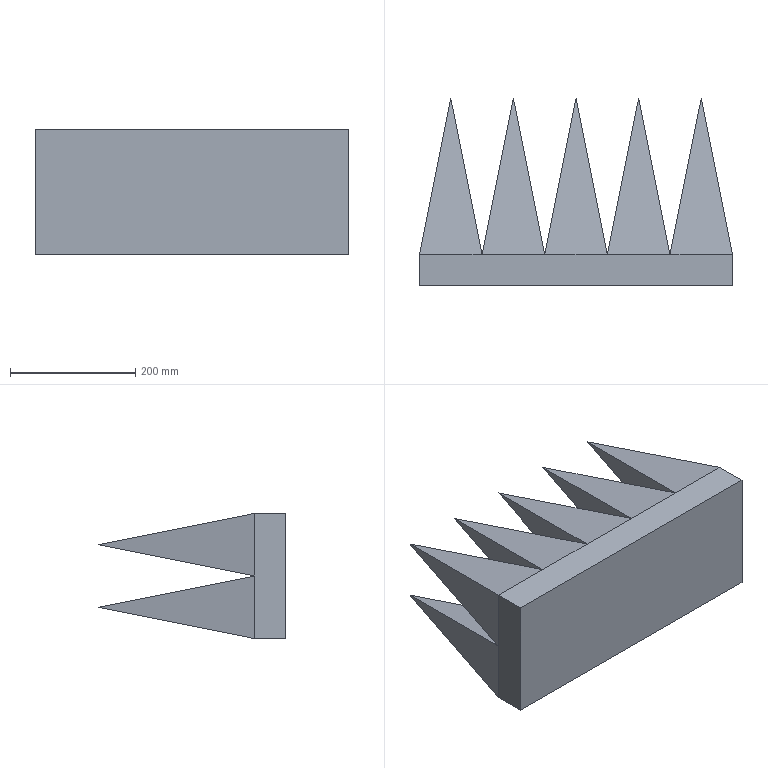Part | SolidWorks | features LPattern 2, Blend 1, Extrusion 1, ICE 1 | 1 solid | 45 faces | box 500 x 300 x 200 mm | volume 13333333 mm3 | plane 45
STEP:
#1=CARTESIAN_POINT('',(250.,50.,-50.));
#2=VERTEX_POINT('',#1);
#3=CARTESIAN_POINT('',(250.,50.,-150.));
#4=VERTEX_POINT('',#3);
#5=CARTESIAN_POINT('',(250.,50.,-50.));
#6=CARTESIAN_POINT('',(250.,50.,-83.333));
#7=CARTESIAN_POINT('',(250.,50.,-116.667));
#8=CARTESIAN_POINT('',(250.,50.,-150.));
#9=B_SPLINE_CURVE_WITH_KNOTS('',3,(#5,#6,#7,#8),.UNSPECIFIED.,.F.,.F.,(4,4),(0.,1.),.UNSPECIFIED.);
#10=EDGE_CURVE('',#2,#4,#9,.T.);
#11=ORIENTED_EDGE('',*,*,#10,.F.);
#12=CARTESIAN_POINT('',(250.,0.,-50.));
#13=VERTEX_POINT('',#12);
#14=CARTESIAN_POINT('',(250.,-0.000025,-50.));
#15=DIRECTION('',(0.,1.,0.));
#16=VECTOR('',#15,1000.);
#17=LINE('',#14,#16);
#18=EDGE_CURVE('',#13,#2,#17,.T.);
#19=ORIENTED_EDGE('',*,*,#18,.F.);
#20=CARTESIAN_POINT('',(250.,0.,-250.));
#21=VERTEX_POINT('',#20);
#22=CARTESIAN_POINT('',(250.,0.,-250.));
#23=DIRECTION('',(0.,0.,-1.));
#24=VECTOR('',#23,1000.);
#25=LINE('',#22,#24);
#26=EDGE_CURVE('',#13,#21,#25,.T.);
#27=ORIENTED_EDGE('',*,*,#26,.T.);
#28=CARTESIAN_POINT('',(250.,50.,-250.));
#29=VERTEX_POINT('',#28);
#30=CARTESIAN_POINT('',(250.,50.,-250.));
#31=DIRECTION('',(0.,-1.,0.));
#32=VECTOR('',#31,1000.);
#33=LINE('',#30,#32);
#34=EDGE_CURVE('',#29,#21,#33,.T.);
#35=ORIENTED_EDGE('',*,*,#34,.F.);
#36=CARTESIAN_POINT('',(250.,50.,-150.));
#37=CARTESIAN_POINT('',(250.,50.,-183.333));
#38=CARTESIAN_POINT('',(250.,50.,-216.667));
#39=CARTESIAN_POINT('',(250.,50.,-250.));
#40=B_SPLINE_CURVE_WITH_KNOTS('',3,(#36,#37,#38,#39),.UNSPECIFIED.,.F.,.F.,(4,4),(0.,1.),.UNSPECIFIED.);
#41=EDGE_CURVE('',#4,#29,#40,.T.);
#42=ORIENTED_EDGE('',*,*,#41,.F.);
#43=EDGE_LOOP('',(#11,#19,#27,#35,#42));
#44=FACE_OUTER_BOUND('',#43,.T.);
#45=CARTESIAN_POINT('',(250.,50.,-250.));
#46=DIRECTION('',(-1.,0.,0.));
#47=DIRECTION('',(0.,0.,1.));
#48=AXIS2_PLACEMENT_3D('',#45,#46,#47);
#49=PLANE('',#48);
#50=ADVANCED_FACE('',(#44),#49,.F.);
#51=CARTESIAN_POINT('',(-250.,0.,-250.));
#52=VERTEX_POINT('',#51);
#53=CARTESIAN_POINT('',(-250.,0.,-250.));
#54=DIRECTION('',(-1.,0.,0.));
#55=VECTOR('',#54,1000.);
#56=LINE('',#53,#55);
#57=EDGE_CURVE('',#21,#52,#56,.T.);
#58=ORIENTED_EDGE('',*,*,#57,.T.);
#59=CARTESIAN_POINT('',(-250.,50.,-250.));
#60=VERTEX_POINT('',#59);
#61=CARTESIAN_POINT('',(-250.,50.,-250.));
#62=DIRECTION('',(0.,-1.,0.));
#63=VECTOR('',#62,1000.);
#64=LINE('',#61,#63);
#65=EDGE_CURVE('',#60,#52,#64,.T.);
#66=ORIENTED_EDGE('',*,*,#65,.F.);
#67=CARTESIAN_POINT('',(-150.,50.,-250.));
#68=VERTEX_POINT('',#67);
#69=CARTESIAN_POINT('',(-150.,50.,-250.));
#70=CARTESIAN_POINT('',(-183.333,50.,-250.));
#71=CARTESIAN_POINT('',(-216.667,50.,-250.));
#72=CARTESIAN_POINT('',(-250.,50.,-250.));
#73=B_SPLINE_CURVE_WITH_KNOTS('',3,(#69,#70,#71,#72),.UNSPECIFIED.,.F.,.F.,(4,4),(0.,1.),.UNSPECIFIED.);
#74=EDGE_CURVE('',#68,#60,#73,.T.);
#75=ORIENTED_EDGE('',*,*,#74,.F.);
#76=CARTESIAN_POINT('',(-50.,50.,-250.));
#77=VERTEX_POINT('',#76);
#78=CARTESIAN_POINT('',(-150.,50.,-250.));
#79=DIRECTION('',(-1.,0.,0.));
#80=VECTOR('',#79,1000.);
#81=LINE('',#78,#80);
#82=EDGE_CURVE('',#77,#68,#81,.T.);
#83=ORIENTED_EDGE('',*,*,#82,.F.);
#84=CARTESIAN_POINT('',(50.,50.,-250.));
#85=VERTEX_POINT('',#84);
#86=CARTESIAN_POINT('',(-50.,50.,-250.));
#87=DIRECTION('',(-1.,0.,0.));
#88=VECTOR('',#87,1000.);
#89=LINE('',#86,#88);
#90=EDGE_CURVE('',#85,#77,#89,.T.);
#91=ORIENTED_EDGE('',*,*,#90,.F.);
#92=CARTESIAN_POINT('',(150.,50.,-250.));
#93=VERTEX_POINT('',#92);
#94=CARTESIAN_POINT('',(50.,50.,-250.));
#95=DIRECTION('',(-1.,0.,0.));
#96=VECTOR('',#95,1000.);
#97=LINE('',#94,#96);
#98=EDGE_CURVE('',#93,#85,#97,.T.);
#99=ORIENTED_EDGE('',*,*,#98,.F.);
#100=CARTESIAN_POINT('',(250.,50.,-250.));
#101=CARTESIAN_POINT('',(216.667,50.,-250.));
#102=CARTESIAN_POINT('',(183.333,50.,-250.));
#103=CARTESIAN_POINT('',(150.,50.,-250.));
#104=B_SPLINE_CURVE_WITH_KNOTS('',3,(#100,#101,#102,#103),.UNSPECIFIED.,.F.,.F.,(4,4),(0.,1.),.UNSPECIFIED.);
#105=EDGE_CURVE('',#29,#93,#104,.T.);
#106=ORIENTED_EDGE('',*,*,#105,.F.);
#107=ORIENTED_EDGE('',*,*,#34,.T.);
#108=EDGE_LOOP('',(#58,#66,#75,#83,#91,#99,#106,#107));
#109=FACE_OUTER_BOUND('',#108,.T.);
#110=CARTESIAN_POINT('',(-250.,50.,-250.));
#111=DIRECTION('',(0.,0.,1.));
#112=DIRECTION('',(1.,0.,0.));
#113=AXIS2_PLACEMENT_3D('',#110,#111,#112);
#114=PLANE('',#113);
#115=ADVANCED_FACE('',(#109),#114,.F.);
#116=CARTESIAN_POINT('',(-250.,0.,-50.));
#117=VERTEX_POINT('',#116);
#118=CARTESIAN_POINT('',(-250.,0.,-250.));
#119=DIRECTION('',(0.,0.,1.));
#120=VECTOR('',#119,1000.);
#121=LINE('',#118,#120);
#122=EDGE_CURVE('',#52,#117,#121,.T.);
#123=ORIENTED_EDGE('',*,*,#122,.T.);
#124=CARTESIAN_POINT('',(-250.,50.,-50.));
#125=VERTEX_POINT('',#124);
#126=CARTESIAN_POINT('',(-250.,-0.000025,-50.));
#127=DIRECTION('',(0.,1.,0.));
#128=VECTOR('',#127,1000.);
#129=LINE('',#126,#128);
#130=EDGE_CURVE('',#117,#125,#129,.T.);
#131=ORIENTED_EDGE('',*,*,#130,.T.);
#132=CARTESIAN_POINT('',(-250.,50.,-150.));
#133=VERTEX_POINT('',#132);
#134=CARTESIAN_POINT('',(-250.,50.,-50.));
#135=DIRECTION('',(0.,0.,1.));
#136=VECTOR('',#135,1000.);
#137=LINE('',#134,#136);
#138=EDGE_CURVE('',#133,#125,#137,.T.);
#139=ORIENTED_EDGE('',*,*,#138,.F.);
#140=CARTESIAN_POINT('',(-250.,50.,-250.));
#141=CARTESIAN_POINT('',(-250.,50.,-216.667));
#142=CARTESIAN_POINT('',(-250.,50.,-183.333));
#143=CARTESIAN_POINT('',(-250.,50.,-150.));
#144=B_SPLINE_CURVE_WITH_KNOTS('',3,(#140,#141,#142,#143),.UNSPECIFIED.,.F.,.F.,(4,4),(0.,1.),.UNSPECIFIED.);
#145=EDGE_CURVE('',#60,#133,#144,.T.);
#146=ORIENTED_EDGE('',*,*,#145,.F.);
#147=ORIENTED_EDGE('',*,*,#65,.T.);
#148=EDGE_LOOP('',(#123,#131,#139,#146,#147));
#149=FACE_OUTER_BOUND('',#148,.T.);
#150=CARTESIAN_POINT('',(-250.,50.,-250.));
#151=DIRECTION('',(1.,0.,0.));
#152=DIRECTION('',(0.,0.,-1.));
#153=AXIS2_PLACEMENT_3D('',#150,#151,#152);
#154=PLANE('',#153);
#155=ADVANCED_FACE('',(#149),#154,.F.);
#156=ORIENTED_EDGE('',*,*,#26,.F.);
#157=CARTESIAN_POINT('',(0.,0.,-50.));
#158=DIRECTION('',(-1.,0.,0.));
#159=VECTOR('',#158,1000.);
#160=LINE('',#157,#159);
#161=EDGE_CURVE('',#13,#117,#160,.T.);
#162=ORIENTED_EDGE('',*,*,#161,.T.);
#163=ORIENTED_EDGE('',*,*,#122,.F.);
#164=ORIENTED_EDGE('',*,*,#57,.F.);
#165=EDGE_LOOP('',(#156,#162,#163,#164));
#166=FACE_OUTER_BOUND('',#165,.T.);
#167=CARTESIAN_POINT('',(0.,0.,0.));
#168=DIRECTION('',(0.,1.,0.));
#169=DIRECTION('',(0.,0.,1.));
#170=AXIS2_PLACEMENT_3D('',#167,#168,#169);
#171=PLANE('',#170);
#172=ADVANCED_FACE('',(#166),#171,.F.);
#173=CARTESIAN_POINT('',(-200.,300.,-100.));
#174=VERTEX_POINT('',#173);
#175=CARTESIAN_POINT('',(-150.,50.,-50.));
#176=VERTEX_POINT('',#175);
#177=CARTESIAN_POINT('',(-200.,300.,-100.));
#178=DIRECTION('',(0.1925,-0.9623,0.1925));
#179=VECTOR('',#178,1000.);
#180=LINE('',#177,#179);
#181=EDGE_CURVE('',#174,#176,#180,.T.);
#182=ORIENTED_EDGE('',*,*,#181,.T.);
#183=CARTESIAN_POINT('',(-150.,50.,-150.));
#184=VERTEX_POINT('',#183);
#185=CARTESIAN_POINT('',(-150.,50.,-50.));
#186=CARTESIAN_POINT('',(-150.,50.,-83.333));
#187=CARTESIAN_POINT('',(-150.,50.,-116.667));
#188=CARTESIAN_POINT('',(-150.,50.,-150.));
#189=B_SPLINE_CURVE_WITH_KNOTS('',3,(#185,#186,#187,#188),.UNSPECIFIED.,.F.,.F.,(4,4),(0.,1.),.UNSPECIFIED.);
#190=EDGE_CURVE('',#176,#184,#189,.T.);
#191=ORIENTED_EDGE('',*,*,#190,.T.);
#192=CARTESIAN_POINT('',(-200.,300.,-100.));
#193=DIRECTION('',(0.1925,-0.9623,-0.1925));
#194=VECTOR('',#193,1000.);
#195=LINE('',#192,#194);
#196=EDGE_CURVE('',#174,#184,#195,.T.);
#197=ORIENTED_EDGE('',*,*,#196,.F.);
#198=EDGE_LOOP('',(#182,#191,#197));
#199=FACE_OUTER_BOUND('',#198,.T.);
#200=CARTESIAN_POINT('',(-134.615,-26.923,-300.));
#201=DIRECTION('',(0.9806,0.1961,0.));
#202=DIRECTION('',(-0.1961,0.9806,0.));
#203=AXIS2_PLACEMENT_3D('',#200,#201,#202);
#204=PLANE('',#203);
#205=ADVANCED_FACE('',(#199),#204,.T.);
#206=ORIENTED_EDGE('',*,*,#196,.T.);
#207=CARTESIAN_POINT('',(-150.,50.,-150.));
#208=CARTESIAN_POINT('',(-183.333,50.,-150.));
#209=CARTESIAN_POINT('',(-216.667,50.,-150.));
#210=CARTESIAN_POINT('',(-250.,50.,-150.));
#211=B_SPLINE_CURVE_WITH_KNOTS('',3,(#207,#208,#209,#210),.UNSPECIFIED.,.F.,.F.,(4,4),(0.,1.),.UNSPECIFIED.);
#212=EDGE_CURVE('',#184,#133,#211,.T.);
#213=ORIENTED_EDGE('',*,*,#212,.T.);
#214=CARTESIAN_POINT('',(-200.,300.,-100.));
#215=DIRECTION('',(-0.1925,-0.9623,-0.1925));
#216=VECTOR('',#215,1000.);
#217=LINE('',#214,#216);
#218=EDGE_CURVE('',#174,#133,#217,.T.);
#219=ORIENTED_EDGE('',*,*,#218,.F.);
#220=EDGE_LOOP('',(#206,#213,#219));
#221=FACE_OUTER_BOUND('',#220,.T.);
#222=CARTESIAN_POINT('',(0.,-26.923,-165.385));
#223=DIRECTION('',(0.,0.1961,-0.9806));
#224=DIRECTION('',(0.,0.9806,0.1961));
#225=AXIS2_PLACEMENT_3D('',#222,#223,#224);
#226=PLANE('',#225);
#227=ADVANCED_FACE('',(#221),#226,.T.);
#228=CARTESIAN_POINT('',(-200.,300.,-100.));
#229=DIRECTION('',(-0.1925,-0.9623,0.1925));
#230=VECTOR('',#229,1000.);
#231=LINE('',#228,#230);
#232=EDGE_CURVE('',#174,#125,#231,.T.);
#233=ORIENTED_EDGE('',*,*,#232,.T.);
#234=CARTESIAN_POINT('',(-150.,50.,-50.));
#235=CARTESIAN_POINT('',(-183.333,50.,-50.));
#236=CARTESIAN_POINT('',(-216.667,50.,-50.));
#237=CARTESIAN_POINT('',(-250.,50.,-50.));
#238=B_SPLINE_CURVE_WITH_KNOTS('',3,(#234,#235,#236,#237),.UNSPECIFIED.,.F.,.F.,(4,4),(0.,1.),.UNSPECIFIED.);
#239=EDGE_CURVE('',#176,#125,#238,.T.);
#240=ORIENTED_EDGE('',*,*,#239,.F.);
#241=ORIENTED_EDGE('',*,*,#181,.F.);
#242=EDGE_LOOP('',(#233,#240,#241));
#243=FACE_OUTER_BOUND('',#242,.T.);
#244=CARTESIAN_POINT('',(0.,50.,-50.));
#245=DIRECTION('',(0.,0.1961,0.9806));
#246=DIRECTION('',(0.,-0.9806,0.1961));
#247=AXIS2_PLACEMENT_3D('',#244,#245,#246);
#248=PLANE('',#247);
#249=ADVANCED_FACE('',(#243),#248,.T.);
#250=ORIENTED_EDGE('',*,*,#218,.T.);
#251=ORIENTED_EDGE('',*,*,#138,.T.);
#252=ORIENTED_EDGE('',*,*,#232,.F.);
#253=EDGE_LOOP('',(#250,#251,#252));
#254=FACE_OUTER_BOUND('',#253,.T.);
#255=CARTESIAN_POINT('',(-250.,50.,-300.));
#256=DIRECTION('',(-0.9806,0.1961,0.));
#257=DIRECTION('',(-0.1961,-0.9806,0.));
#258=AXIS2_PLACEMENT_3D('',#255,#256,#257);
#259=PLANE('',#258);
#260=ADVANCED_FACE('',(#254),#259,.T.);
#261=CARTESIAN_POINT('',(-100.,300.,-100.));
#262=VERTEX_POINT('',#261);
#263=CARTESIAN_POINT('',(-50.,50.,-50.));
#264=VERTEX_POINT('',#263);
#265=CARTESIAN_POINT('',(-100.,300.,-100.));
#266=DIRECTION('',(0.1925,-0.9623,0.1925));
#267=VECTOR('',#266,1000.);
#268=LINE('',#265,#267);
#269=EDGE_CURVE('',#262,#264,#268,.T.);
#270=ORIENTED_EDGE('',*,*,#269,.T.);
#271=CARTESIAN_POINT('',(-50.,50.,-150.));
#272=VERTEX_POINT('',#271);
#273=CARTESIAN_POINT('',(-50.,50.,-50.));
#274=CARTESIAN_POINT('',(-50.,50.,-83.333));
#275=CARTESIAN_POINT('',(-50.,50.,-116.667));
#276=CARTESIAN_POINT('',(-50.,50.,-150.));
#277=B_SPLINE_CURVE_WITH_KNOTS('',3,(#273,#274,#275,#276),.UNSPECIFIED.,.F.,.F.,(4,4),(0.,1.),.UNSPECIFIED.);
#278=EDGE_CURVE('',#264,#272,#277,.T.);
#279=ORIENTED_EDGE('',*,*,#278,.T.);
#280=CARTESIAN_POINT('',(-100.,300.,-100.));
#281=DIRECTION('',(0.1925,-0.9623,-0.1925));
#282=VECTOR('',#281,1000.);
#283=LINE('',#280,#282);
#284=EDGE_CURVE('',#262,#272,#283,.T.);
#285=ORIENTED_EDGE('',*,*,#284,.F.);
#286=EDGE_LOOP('',(#270,#279,#285));
#287=FACE_OUTER_BOUND('',#286,.T.);
#288=CARTESIAN_POINT('',(-34.615,-26.923,-300.));
#289=DIRECTION('',(0.9806,0.1961,0.));
#290=DIRECTION('',(-0.1961,0.9806,0.));
#291=AXIS2_PLACEMENT_3D('',#288,#289,#290);
#292=PLANE('',#291);
#293=ADVANCED_FACE('',(#287),#292,.T.);
#294=ORIENTED_EDGE('',*,*,#284,.T.);
#295=CARTESIAN_POINT('',(-50.,50.,-150.));
#296=CARTESIAN_POINT('',(-83.333,50.,-150.));
#297=CARTESIAN_POINT('',(-116.667,50.,-150.));
#298=CARTESIAN_POINT('',(-150.,50.,-150.));
#299=B_SPLINE_CURVE_WITH_KNOTS('',3,(#295,#296,#297,#298),.UNSPECIFIED.,.F.,.F.,(4,4),(0.,1.),.UNSPECIFIED.);
#300=EDGE_CURVE('',#272,#184,#299,.T.);
#301=ORIENTED_EDGE('',*,*,#300,.T.);
#302=CARTESIAN_POINT('',(-100.,300.,-100.));
#303=DIRECTION('',(-0.1925,-0.9623,-0.1925));
#304=VECTOR('',#303,1000.);
#305=LINE('',#302,#304);
#306=EDGE_CURVE('',#262,#184,#305,.T.);
#307=ORIENTED_EDGE('',*,*,#306,.F.);
#308=EDGE_LOOP('',(#294,#301,#307));
#309=FACE_OUTER_BOUND('',#308,.T.);
#310=CARTESIAN_POINT('',(100.,-26.923,-165.385));
#311=DIRECTION('',(0.,0.1961,-0.9806));
#312=DIRECTION('',(0.,0.9806,0.1961));
#313=AXIS2_PLACEMENT_3D('',#310,#311,#312);
#314=PLANE('',#313);
#315=ADVANCED_FACE('',(#309),#314,.T.);
#316=CARTESIAN_POINT('',(-100.,300.,-100.));
#317=DIRECTION('',(-0.1925,-0.9623,0.1925));
#318=VECTOR('',#317,1000.);
#319=LINE('',#316,#318);
#320=EDGE_CURVE('',#262,#176,#319,.T.);
#321=ORIENTED_EDGE('',*,*,#320,.T.);
#322=CARTESIAN_POINT('',(-50.,50.,-50.));
#323=CARTESIAN_POINT('',(-83.333,50.,-50.));
#324=CARTESIAN_POINT('',(-116.667,50.,-50.));
#325=CARTESIAN_POINT('',(-150.,50.,-50.));
#326=B_SPLINE_CURVE_WITH_KNOTS('',3,(#322,#323,#324,#325),.UNSPECIFIED.,.F.,.F.,(4,4),(0.,1.),.UNSPECIFIED.);
#327=EDGE_CURVE('',#264,#176,#326,.T.);
#328=ORIENTED_EDGE('',*,*,#327,.F.);
#329=ORIENTED_EDGE('',*,*,#269,.F.);
#330=EDGE_LOOP('',(#321,#328,#329));
#331=FACE_OUTER_BOUND('',#330,.T.);
#332=CARTESIAN_POINT('',(100.,50.,-50.));
#333=DIRECTION('',(0.,0.1961,0.9806));
#334=DIRECTION('',(0.,-0.9806,0.1961));
#335=AXIS2_PLACEMENT_3D('',#332,#333,#334);
#336=PLANE('',#335);
#337=ADVANCED_FACE('',(#331),#336,.T.);
#338=ORIENTED_EDGE('',*,*,#306,.T.);
#339=ORIENTED_EDGE('',*,*,#190,.F.);
#340=ORIENTED_EDGE('',*,*,#320,.F.);
#341=EDGE_LOOP('',(#338,#339,#340));
#342=FACE_OUTER_BOUND('',#341,.T.);
#343=CARTESIAN_POINT('',(-150.,50.,-300.));
#344=DIRECTION('',(-0.9806,0.1961,0.));
#345=DIRECTION('',(-0.1961,-0.9806,0.));
#346=AXIS2_PLACEMENT_3D('',#343,#344,#345);
#347=PLANE('',#346);
#348=ADVANCED_FACE('',(#342),#347,.T.);
#349=CARTESIAN_POINT('',(0.,300.,-100.));
#350=VERTEX_POINT('',#349);
#351=CARTESIAN_POINT('',(50.,50.,-50.));
#352=VERTEX_POINT('',#351);
#353=CARTESIAN_POINT('',(0.,300.,-100.));
#354=DIRECTION('',(0.1925,-0.9623,0.1925));
#355=VECTOR('',#354,1000.);
#356=LINE('',#353,#355);
#357=EDGE_CURVE('',#350,#352,#356,.T.);
#358=ORIENTED_EDGE('',*,*,#357,.T.);
#359=CARTESIAN_POINT('',(50.,50.,-150.));
#360=VERTEX_POINT('',#359);
#361=CARTESIAN_POINT('',(50.,50.,-50.));
#362=CARTESIAN_POINT('',(50.,50.,-83.333));
#363=CARTESIAN_POINT('',(50.,50.,-116.667));
#364=CARTESIAN_POINT('',(50.,50.,-150.));
#365=B_SPLINE_CURVE_WITH_KNOTS('',3,(#361,#362,#363,#364),.UNSPECIFIED.,.F.,.F.,(4,4),(0.,1.),.UNSPECIFIED.);
#366=EDGE_CURVE('',#352,#360,#365,.T.);
#367=ORIENTED_EDGE('',*,*,#366,.T.);
#368=CARTESIAN_POINT('',(0.,300.,-100.));
#369=DIRECTION('',(0.1925,-0.9623,-0.1925));
#370=VECTOR('',#369,1000.);
#371=LINE('',#368,#370);
#372=EDGE_CURVE('',#350,#360,#371,.T.);
#373=ORIENTED_EDGE('',*,*,#372,.F.);
#374=EDGE_LOOP('',(#358,#367,#373));
#375=FACE_OUTER_BOUND('',#374,.T.);
#376=CARTESIAN_POINT('',(65.385,-26.923,-300.));
#377=DIRECTION('',(0.9806,0.1961,0.));
#378=DIRECTION('',(-0.1961,0.9806,0.));
#379=AXIS2_PLACEMENT_3D('',#376,#377,#378);
#380=PLANE('',#379);
#381=ADVANCED_FACE('',(#375),#380,.T.);
#382=ORIENTED_EDGE('',*,*,#372,.T.);
#383=CARTESIAN_POINT('',(50.,50.,-150.));
#384=CARTESIAN_POINT('',(16.667,50.,-150.));
#385=CARTESIAN_POINT('',(-16.667,50.,-150.));
#386=CARTESIAN_POINT('',(-50.,50.,-150.));
#387=B_SPLINE_CURVE_WITH_KNOTS('',3,(#383,#384,#385,#386),.UNSPECIFIED.,.F.,.F.,(4,4),(0.,1.),.UNSPECIFIED.);
#388=EDGE_CURVE('',#360,#272,#387,.T.);
#389=ORIENTED_EDGE('',*,*,#388,.T.);
#390=CARTESIAN_POINT('',(0.,300.,-100.));
#391=DIRECTION('',(-0.1925,-0.9623,-0.1925));
#392=VECTOR('',#391,1000.);
#393=LINE('',#390,#392);
#394=EDGE_CURVE('',#350,#272,#393,.T.);
#395=ORIENTED_EDGE('',*,*,#394,.F.);
#396=EDGE_LOOP('',(#382,#389,#395));
#397=FACE_OUTER_BOUND('',#396,.T.);
#398=CARTESIAN_POINT('',(200.,-26.923,-165.385));
#399=DIRECTION('',(0.,0.1961,-0.9806));
#400=DIRECTION('',(0.,0.9806,0.1961));
#401=AXIS2_PLACEMENT_3D('',#398,#399,#400);
#402=PLANE('',#401);
#403=ADVANCED_FACE('',(#397),#402,.T.);
#404=CARTESIAN_POINT('',(0.,300.,-100.));
#405=DIRECTION('',(-0.1925,-0.9623,0.1925));
#406=VECTOR('',#405,1000.);
#407=LINE('',#404,#406);
#408=EDGE_CURVE('',#350,#264,#407,.T.);
#409=ORIENTED_EDGE('',*,*,#408,.T.);
#410=CARTESIAN_POINT('',(50.,50.,-50.));
#411=CARTESIAN_POINT('',(16.667,50.,-50.));
#412=CARTESIAN_POINT('',(-16.667,50.,-50.));
#413=CARTESIAN_POINT('',(-50.,50.,-50.));
#414=B_SPLINE_CURVE_WITH_KNOTS('',3,(#410,#411,#412,#413),.UNSPECIFIED.,.F.,.F.,(4,4),(0.,1.),.UNSPECIFIED.);
#415=EDGE_CURVE('',#352,#264,#414,.T.);
#416=ORIENTED_EDGE('',*,*,#415,.F.);
#417=ORIENTED_EDGE('',*,*,#357,.F.);
#418=EDGE_LOOP('',(#409,#416,#417));
#419=FACE_OUTER_BOUND('',#418,.T.);
#420=CARTESIAN_POINT('',(200.,50.,-50.));
#421=DIRECTION('',(0.,0.1961,0.9806));
#422=DIRECTION('',(0.,-0.9806,0.1961));
#423=AXIS2_PLACEMENT_3D('',#420,#421,#422);
#424=PLANE('',#423);
#425=ADVANCED_FACE('',(#419),#424,.T.);
#426=ORIENTED_EDGE('',*,*,#394,.T.);
#427=ORIENTED_EDGE('',*,*,#278,.F.);
#428=ORIENTED_EDGE('',*,*,#408,.F.);
#429=EDGE_LOOP('',(#426,#427,#428));
#430=FACE_OUTER_BOUND('',#429,.T.);
#431=CARTESIAN_POINT('',(-50.,50.,-300.));
#432=DIRECTION('',(-0.9806,0.1961,0.));
#433=DIRECTION('',(-0.1961,-0.9806,0.));
#434=AXIS2_PLACEMENT_3D('',#431,#432,#433);
#435=PLANE('',#434);
#436=ADVANCED_FACE('',(#430),#435,.T.);
#437=CARTESIAN_POINT('',(100.,300.,-100.));
#438=VERTEX_POINT('',#437);
#439=CARTESIAN_POINT('',(150.,50.,-50.));
#440=VERTEX_POINT('',#439);
#441=CARTESIAN_POINT('',(100.,300.,-100.));
#442=DIRECTION('',(0.1925,-0.9623,0.1925));
#443=VECTOR('',#442,1000.);
#444=LINE('',#441,#443);
#445=EDGE_CURVE('',#438,#440,#444,.T.);
#446=ORIENTED_EDGE('',*,*,#445,.T.);
#447=CARTESIAN_POINT('',(150.,50.,-150.));
#448=VERTEX_POINT('',#447);
#449=CARTESIAN_POINT('',(150.,50.,-50.));
#450=CARTESIAN_POINT('',(150.,50.,-83.333));
#451=CARTESIAN_POINT('',(150.,50.,-116.667));
#452=CARTESIAN_POINT('',(150.,50.,-150.));
#453=B_SPLINE_CURVE_WITH_KNOTS('',3,(#449,#450,#451,#452),.UNSPECIFIED.,.F.,.F.,(4,4),(0.,1.),.UNSPECIFIED.);
#454=EDGE_CURVE('',#440,#448,#453,.T.);
#455=ORIENTED_EDGE('',*,*,#454,.T.);
#456=CARTESIAN_POINT('',(100.,300.,-100.));
#457=DIRECTION('',(0.1925,-0.9623,-0.1925));
#458=VECTOR('',#457,1000.);
#459=LINE('',#456,#458);
#460=EDGE_CURVE('',#438,#448,#459,.T.);
#461=ORIENTED_EDGE('',*,*,#460,.F.);
#462=EDGE_LOOP('',(#446,#455,#461));
#463=FACE_OUTER_BOUND('',#462,.T.);
#464=CARTESIAN_POINT('',(165.385,-26.923,-300.));
#465=DIRECTION('',(0.9806,0.1961,0.));
#466=DIRECTION('',(-0.1961,0.9806,0.));
#467=AXIS2_PLACEMENT_3D('',#464,#465,#466);
#468=PLANE('',#467);
#469=ADVANCED_FACE('',(#463),#468,.T.);
#470=ORIENTED_EDGE('',*,*,#460,.T.);
#471=CARTESIAN_POINT('',(150.,50.,-150.));
#472=CARTESIAN_POINT('',(116.667,50.,-150.));
#473=CARTESIAN_POINT('',(83.333,50.,-150.));
#474=CARTESIAN_POINT('',(50.,50.,-150.));
#475=B_SPLINE_CURVE_WITH_KNOTS('',3,(#471,#472,#473,#474),.UNSPECIFIED.,.F.,.F.,(4,4),(0.,1.),.UNSPECIFIED.);
#476=EDGE_CURVE('',#448,#360,#475,.T.);
#477=ORIENTED_EDGE('',*,*,#476,.T.);
#478=CARTESIAN_POINT('',(100.,300.,-100.));
#479=DIRECTION('',(-0.1925,-0.9623,-0.1925));
#480=VECTOR('',#479,1000.);
#481=LINE('',#478,#480);
#482=EDGE_CURVE('',#438,#360,#481,.T.);
#483=ORIENTED_EDGE('',*,*,#482,.F.);
#484=EDGE_LOOP('',(#470,#477,#483));
#485=FACE_OUTER_BOUND('',#484,.T.);
#486=CARTESIAN_POINT('',(300.,-26.923,-165.385));
#487=DIRECTION('',(0.,0.1961,-0.9806));
#488=DIRECTION('',(0.,0.9806,0.1961));
#489=AXIS2_PLACEMENT_3D('',#486,#487,#488);
#490=PLANE('',#489);
#491=ADVANCED_FACE('',(#485),#490,.T.);
#492=CARTESIAN_POINT('',(100.,300.,-100.));
#493=DIRECTION('',(-0.1925,-0.9623,0.1925));
#494=VECTOR('',#493,1000.);
#495=LINE('',#492,#494);
#496=EDGE_CURVE('',#438,#352,#495,.T.);
#497=ORIENTED_EDGE('',*,*,#496,.T.);
#498=CARTESIAN_POINT('',(150.,50.,-50.));
#499=CARTESIAN_POINT('',(116.667,50.,-50.));
#500=CARTESIAN_POINT('',(83.333,50.,-50.));
#501=CARTESIAN_POINT('',(50.,50.,-50.));
#502=B_SPLINE_CURVE_WITH_KNOTS('',3,(#498,#499,#500,#501),.UNSPECIFIED.,.F.,.F.,(4,4),(0.,1.),.UNSPECIFIED.);
#503=EDGE_CURVE('',#440,#352,#502,.T.);
#504=ORIENTED_EDGE('',*,*,#503,.F.);
#505=ORIENTED_EDGE('',*,*,#445,.F.);
#506=EDGE_LOOP('',(#497,#504,#505));
#507=FACE_OUTER_BOUND('',#506,.T.);
#508=CARTESIAN_POINT('',(300.,50.,-50.));
#509=DIRECTION('',(0.,0.1961,0.9806));
#510=DIRECTION('',(0.,-0.9806,0.1961));
#511=AXIS2_PLACEMENT_3D('',#508,#509,#510);
#512=PLANE('',#511);
#513=ADVANCED_FACE('',(#507),#512,.T.);
#514=ORIENTED_EDGE('',*,*,#482,.T.);
#515=ORIENTED_EDGE('',*,*,#366,.F.);
#516=ORIENTED_EDGE('',*,*,#496,.F.);
#517=EDGE_LOOP('',(#514,#515,#516));
#518=FACE_OUTER_BOUND('',#517,.T.);
#519=CARTESIAN_POINT('',(50.,50.,-300.));
#520=DIRECTION('',(-0.9806,0.1961,0.));
#521=DIRECTION('',(-0.1961,-0.9806,0.));
#522=AXIS2_PLACEMENT_3D('',#519,#520,#521);
#523=PLANE('',#522);
#524=ADVANCED_FACE('',(#518),#523,.T.);
#525=CARTESIAN_POINT('',(200.,300.,-100.));
#526=VERTEX_POINT('',#525);
#527=CARTESIAN_POINT('',(200.,300.,-100.));
#528=DIRECTION('',(0.1925,-0.9623,0.1925));
#529=VECTOR('',#528,1000.);
#530=LINE('',#527,#529);
#531=EDGE_CURVE('',#526,#2,#530,.T.);
#532=ORIENTED_EDGE('',*,*,#531,.T.);
#533=ORIENTED_EDGE('',*,*,#10,.T.);
#534=CARTESIAN_POINT('',(200.,300.,-100.));
#535=DIRECTION('',(0.1925,-0.9623,-0.1925));
#536=VECTOR('',#535,1000.);
#537=LINE('',#534,#536);
#538=EDGE_CURVE('',#526,#4,#537,.T.);
#539=ORIENTED_EDGE('',*,*,#538,.F.);
#540=EDGE_LOOP('',(#532,#533,#539));
#541=FACE_OUTER_BOUND('',#540,.T.);
#542=CARTESIAN_POINT('',(265.385,-26.923,-300.));
#543=DIRECTION('',(0.9806,0.1961,0.));
#544=DIRECTION('',(-0.1961,0.9806,0.));
#545=AXIS2_PLACEMENT_3D('',#542,#543,#544);
#546=PLANE('',#545);
#547=ADVANCED_FACE('',(#541),#546,.T.);
#548=ORIENTED_EDGE('',*,*,#538,.T.);
#549=CARTESIAN_POINT('',(250.,50.,-150.));
#550=CARTESIAN_POINT('',(216.667,50.,-150.));
#551=CARTESIAN_POINT('',(183.333,50.,-150.));
#552=CARTESIAN_POINT('',(150.,50.,-150.));
#553=B_SPLINE_CURVE_WITH_KNOTS('',3,(#549,#550,#551,#552),.UNSPECIFIED.,.F.,.F.,(4,4),(0.,1.),.UNSPECIFIED.);
#554=EDGE_CURVE('',#4,#448,#553,.T.);
#555=ORIENTED_EDGE('',*,*,#554,.T.);
#556=CARTESIAN_POINT('',(200.,300.,-100.));
#557=DIRECTION('',(-0.1925,-0.9623,-0.1925));
#558=VECTOR('',#557,1000.);
#559=LINE('',#556,#558);
#560=EDGE_CURVE('',#526,#448,#559,.T.);
#561=ORIENTED_EDGE('',*,*,#560,.F.);
#562=EDGE_LOOP('',(#548,#555,#561));
#563=FACE_OUTER_BOUND('',#562,.T.);
#564=CARTESIAN_POINT('',(400.,-26.923,-165.385));
#565=DIRECTION('',(0.,0.1961,-0.9806));
#566=DIRECTION('',(0.,0.9806,0.1961));
#567=AXIS2_PLACEMENT_3D('',#564,#565,#566);
#568=PLANE('',#567);
#569=ADVANCED_FACE('',(#563),#568,.T.);
#570=CARTESIAN_POINT('',(200.,300.,-100.));
#571=DIRECTION('',(-0.1925,-0.9623,0.1925));
#572=VECTOR('',#571,1000.);
#573=LINE('',#570,#572);
#574=EDGE_CURVE('',#526,#440,#573,.T.);
#575=ORIENTED_EDGE('',*,*,#574,.T.);
#576=CARTESIAN_POINT('',(250.,50.,-50.));
#577=CARTESIAN_POINT('',(216.667,50.,-50.));
#578=CARTESIAN_POINT('',(183.333,50.,-50.));
#579=CARTESIAN_POINT('',(150.,50.,-50.));
#580=B_SPLINE_CURVE_WITH_KNOTS('',3,(#576,#577,#578,#579),.UNSPECIFIED.,.F.,.F.,(4,4),(0.,1.),.UNSPECIFIED.);
#581=EDGE_CURVE('',#2,#440,#580,.T.);
#582=ORIENTED_EDGE('',*,*,#581,.F.);
#583=ORIENTED_EDGE('',*,*,#531,.F.);
#584=EDGE_LOOP('',(#575,#582,#583));
#585=FACE_OUTER_BOUND('',#584,.T.);
#586=CARTESIAN_POINT('',(400.,50.,-50.));
#587=DIRECTION('',(0.,0.1961,0.9806));
#588=DIRECTION('',(0.,-0.9806,0.1961));
#589=AXIS2_PLACEMENT_3D('',#586,#587,#588);
#590=PLANE('',#589);
#591=ADVANCED_FACE('',(#585),#590,.T.);
#592=ORIENTED_EDGE('',*,*,#560,.T.);
#593=ORIENTED_EDGE('',*,*,#454,.F.);
#594=ORIENTED_EDGE('',*,*,#574,.F.);
#595=EDGE_LOOP('',(#592,#593,#594));
#596=FACE_OUTER_BOUND('',#595,.T.);
#597=CARTESIAN_POINT('',(150.,50.,-300.));
#598=DIRECTION('',(-0.9806,0.1961,0.));
#599=DIRECTION('',(-0.1961,-0.9806,0.));
#600=AXIS2_PLACEMENT_3D('',#597,#598,#599);
#601=PLANE('',#600);
#602=ADVANCED_FACE('',(#596),#601,.T.);
#603=CARTESIAN_POINT('',(-200.,300.,-200.));
#604=VERTEX_POINT('',#603);
#605=CARTESIAN_POINT('',(-200.,300.,-200.));
#606=DIRECTION('',(0.1925,-0.9623,0.1925));
#607=VECTOR('',#606,1000.);
#608=LINE('',#605,#607);
#609=EDGE_CURVE('',#604,#184,#608,.T.);
#610=ORIENTED_EDGE('',*,*,#609,.T.);
#611=CARTESIAN_POINT('',(-150.,50.,-150.));
#612=CARTESIAN_POINT('',(-150.,50.,-183.333));
#613=CARTESIAN_POINT('',(-150.,50.,-216.667));
#614=CARTESIAN_POINT('',(-150.,50.,-250.));
#615=B_SPLINE_CURVE_WITH_KNOTS('',3,(#611,#612,#613,#614),.UNSPECIFIED.,.F.,.F.,(4,4),(0.,1.),.UNSPECIFIED.);
#616=EDGE_CURVE('',#184,#68,#615,.T.);
#617=ORIENTED_EDGE('',*,*,#616,.T.);
#618=CARTESIAN_POINT('',(-200.,300.,-200.));
#619=DIRECTION('',(0.1925,-0.9623,-0.1925));
#620=VECTOR('',#619,1000.);
#621=LINE('',#618,#620);
#622=EDGE_CURVE('',#604,#68,#621,.T.);
#623=ORIENTED_EDGE('',*,*,#622,.F.);
#624=EDGE_LOOP('',(#610,#617,#623));
#625=FACE_OUTER_BOUND('',#624,.T.);
#626=CARTESIAN_POINT('',(-134.615,-26.923,-400.));
#627=DIRECTION('',(0.9806,0.1961,0.));
#628=DIRECTION('',(-0.1961,0.9806,0.));
#629=AXIS2_PLACEMENT_3D('',#626,#627,#628);
#630=PLANE('',#629);
#631=ADVANCED_FACE('',(#625),#630,.T.);
#632=ORIENTED_EDGE('',*,*,#622,.T.);
#633=ORIENTED_EDGE('',*,*,#74,.T.);
#634=CARTESIAN_POINT('',(-200.,300.,-200.));
#635=DIRECTION('',(-0.1925,-0.9623,-0.1925));
#636=VECTOR('',#635,1000.);
#637=LINE('',#634,#636);
#638=EDGE_CURVE('',#604,#60,#637,.T.);
#639=ORIENTED_EDGE('',*,*,#638,.F.);
#640=EDGE_LOOP('',(#632,#633,#639));
#641=FACE_OUTER_BOUND('',#640,.T.);
#642=CARTESIAN_POINT('',(0.,-26.923,-265.385));
#643=DIRECTION('',(0.,0.1961,-0.9806));
#644=DIRECTION('',(0.,0.9806,0.1961));
#645=AXIS2_PLACEMENT_3D('',#642,#643,#644);
#646=PLANE('',#645);
#647=ADVANCED_FACE('',(#641),#646,.T.);
#648=CARTESIAN_POINT('',(-200.,300.,-200.));
#649=DIRECTION('',(-0.1925,-0.9623,0.1925));
#650=VECTOR('',#649,1000.);
#651=LINE('',#648,#650);
#652=EDGE_CURVE('',#604,#133,#651,.T.);
#653=ORIENTED_EDGE('',*,*,#652,.T.);
#654=ORIENTED_EDGE('',*,*,#212,.F.);
#655=ORIENTED_EDGE('',*,*,#609,.F.);
#656=EDGE_LOOP('',(#653,#654,#655));
#657=FACE_OUTER_BOUND('',#656,.T.);
#658=CARTESIAN_POINT('',(0.,50.,-150.));
#659=DIRECTION('',(0.,0.1961,0.9806));
#660=DIRECTION('',(0.,-0.9806,0.1961));
#661=AXIS2_PLACEMENT_3D('',#658,#659,#660);
#662=PLANE('',#661);
#663=ADVANCED_FACE('',(#657),#662,.T.);
#664=ORIENTED_EDGE('',*,*,#638,.T.);
#665=ORIENTED_EDGE('',*,*,#145,.T.);
#666=ORIENTED_EDGE('',*,*,#652,.F.);
#667=EDGE_LOOP('',(#664,#665,#666));
#668=FACE_OUTER_BOUND('',#667,.T.);
#669=CARTESIAN_POINT('',(-250.,50.,-400.));
#670=DIRECTION('',(-0.9806,0.1961,0.));
#671=DIRECTION('',(-0.1961,-0.9806,0.));
#672=AXIS2_PLACEMENT_3D('',#669,#670,#671);
#673=PLANE('',#672);
#674=ADVANCED_FACE('',(#668),#673,.T.);
#675=CARTESIAN_POINT('',(-100.,300.,-200.));
#676=VERTEX_POINT('',#675);
#677=CARTESIAN_POINT('',(-100.,300.,-200.));
#678=DIRECTION('',(0.1925,-0.9623,0.1925));
#679=VECTOR('',#678,1000.);
#680=LINE('',#677,#679);
#681=EDGE_CURVE('',#676,#272,#680,.T.);
#682=ORIENTED_EDGE('',*,*,#681,.T.);
#683=CARTESIAN_POINT('',(-50.,50.,-150.));
#684=CARTESIAN_POINT('',(-50.,50.,-183.333));
#685=CARTESIAN_POINT('',(-50.,50.,-216.667));
#686=CARTESIAN_POINT('',(-50.,50.,-250.));
#687=B_SPLINE_CURVE_WITH_KNOTS('',3,(#683,#684,#685,#686),.UNSPECIFIED.,.F.,.F.,(4,4),(0.,1.),.UNSPECIFIED.);
#688=EDGE_CURVE('',#272,#77,#687,.T.);
#689=ORIENTED_EDGE('',*,*,#688,.T.);
#690=CARTESIAN_POINT('',(-100.,300.,-200.));
#691=DIRECTION('',(0.1925,-0.9623,-0.1925));
#692=VECTOR('',#691,1000.);
#693=LINE('',#690,#692);
#694=EDGE_CURVE('',#676,#77,#693,.T.);
#695=ORIENTED_EDGE('',*,*,#694,.F.);
#696=EDGE_LOOP('',(#682,#689,#695));
#697=FACE_OUTER_BOUND('',#696,.T.);
#698=CARTESIAN_POINT('',(-34.615,-26.923,-400.));
#699=DIRECTION('',(0.9806,0.1961,0.));
#700=DIRECTION('',(-0.1961,0.9806,0.));
#701=AXIS2_PLACEMENT_3D('',#698,#699,#700);
#702=PLANE('',#701);
#703=ADVANCED_FACE('',(#697),#702,.T.);
#704=ORIENTED_EDGE('',*,*,#694,.T.);
#705=ORIENTED_EDGE('',*,*,#82,.T.);
#706=CARTESIAN_POINT('',(-100.,300.,-200.));
#707=DIRECTION('',(-0.1925,-0.9623,-0.1925));
#708=VECTOR('',#707,1000.);
#709=LINE('',#706,#708);
#710=EDGE_CURVE('',#676,#68,#709,.T.);
#711=ORIENTED_EDGE('',*,*,#710,.F.);
#712=EDGE_LOOP('',(#704,#705,#711));
#713=FACE_OUTER_BOUND('',#712,.T.);
#714=CARTESIAN_POINT('',(100.,-26.923,-265.385));
#715=DIRECTION('',(0.,0.1961,-0.9806));
#716=DIRECTION('',(0.,0.9806,0.1961));
#717=AXIS2_PLACEMENT_3D('',#714,#715,#716);
#718=PLANE('',#717);
#719=ADVANCED_FACE('',(#713),#718,.T.);
#720=CARTESIAN_POINT('',(-100.,300.,-200.));
#721=DIRECTION('',(-0.1925,-0.9623,0.1925));
#722=VECTOR('',#721,1000.);
#723=LINE('',#720,#722);
#724=EDGE_CURVE('',#676,#184,#723,.T.);
#725=ORIENTED_EDGE('',*,*,#724,.T.);
#726=ORIENTED_EDGE('',*,*,#300,.F.);
#727=ORIENTED_EDGE('',*,*,#681,.F.);
#728=EDGE_LOOP('',(#725,#726,#727));
#729=FACE_OUTER_BOUND('',#728,.T.);
#730=CARTESIAN_POINT('',(100.,50.,-150.));
#731=DIRECTION('',(0.,0.1961,0.9806));
#732=DIRECTION('',(0.,-0.9806,0.1961));
#733=AXIS2_PLACEMENT_3D('',#730,#731,#732);
#734=PLANE('',#733);
#735=ADVANCED_FACE('',(#729),#734,.T.);
#736=ORIENTED_EDGE('',*,*,#710,.T.);
#737=ORIENTED_EDGE('',*,*,#616,.F.);
#738=ORIENTED_EDGE('',*,*,#724,.F.);
#739=EDGE_LOOP('',(#736,#737,#738));
#740=FACE_OUTER_BOUND('',#739,.T.);
#741=CARTESIAN_POINT('',(-150.,50.,-400.));
#742=DIRECTION('',(-0.9806,0.1961,0.));
#743=DIRECTION('',(-0.1961,-0.9806,0.));
#744=AXIS2_PLACEMENT_3D('',#741,#742,#743);
#745=PLANE('',#744);
#746=ADVANCED_FACE('',(#740),#745,.T.);
#747=CARTESIAN_POINT('',(0.,300.,-200.));
#748=VERTEX_POINT('',#747);
#749=CARTESIAN_POINT('',(0.,300.,-200.));
#750=DIRECTION('',(0.1925,-0.9623,0.1925));
#751=VECTOR('',#750,1000.);
#752=LINE('',#749,#751);
#753=EDGE_CURVE('',#748,#360,#752,.T.);
#754=ORIENTED_EDGE('',*,*,#753,.T.);
#755=CARTESIAN_POINT('',(50.,50.,-150.));
#756=CARTESIAN_POINT('',(50.,50.,-183.333));
#757=CARTESIAN_POINT('',(50.,50.,-216.667));
#758=CARTESIAN_POINT('',(50.,50.,-250.));
#759=B_SPLINE_CURVE_WITH_KNOTS('',3,(#755,#756,#757,#758),.UNSPECIFIED.,.F.,.F.,(4,4),(0.,1.),.UNSPECIFIED.);
#760=EDGE_CURVE('',#360,#85,#759,.T.);
#761=ORIENTED_EDGE('',*,*,#760,.T.);
#762=CARTESIAN_POINT('',(0.,300.,-200.));
#763=DIRECTION('',(0.1925,-0.9623,-0.1925));
#764=VECTOR('',#763,1000.);
#765=LINE('',#762,#764);
#766=EDGE_CURVE('',#748,#85,#765,.T.);
#767=ORIENTED_EDGE('',*,*,#766,.F.);
#768=EDGE_LOOP('',(#754,#761,#767));
#769=FACE_OUTER_BOUND('',#768,.T.);
#770=CARTESIAN_POINT('',(65.385,-26.923,-400.));
#771=DIRECTION('',(0.9806,0.1961,0.));
#772=DIRECTION('',(-0.1961,0.9806,0.));
#773=AXIS2_PLACEMENT_3D('',#770,#771,#772);
#774=PLANE('',#773);
#775=ADVANCED_FACE('',(#769),#774,.T.);
#776=ORIENTED_EDGE('',*,*,#766,.T.);
#777=ORIENTED_EDGE('',*,*,#90,.T.);
#778=CARTESIAN_POINT('',(0.,300.,-200.));
#779=DIRECTION('',(-0.1925,-0.9623,-0.1925));
#780=VECTOR('',#779,1000.);
#781=LINE('',#778,#780);
#782=EDGE_CURVE('',#748,#77,#781,.T.);
#783=ORIENTED_EDGE('',*,*,#782,.F.);
#784=EDGE_LOOP('',(#776,#777,#783));
#785=FACE_OUTER_BOUND('',#784,.T.);
#786=CARTESIAN_POINT('',(200.,-26.923,-265.385));
#787=DIRECTION('',(0.,0.1961,-0.9806));
#788=DIRECTION('',(0.,0.9806,0.1961));
#789=AXIS2_PLACEMENT_3D('',#786,#787,#788);
#790=PLANE('',#789);
#791=ADVANCED_FACE('',(#785),#790,.T.);
#792=CARTESIAN_POINT('',(0.,300.,-200.));
#793=DIRECTION('',(-0.1925,-0.9623,0.1925));
#794=VECTOR('',#793,1000.);
#795=LINE('',#792,#794);
#796=EDGE_CURVE('',#748,#272,#795,.T.);
#797=ORIENTED_EDGE('',*,*,#796,.T.);
#798=ORIENTED_EDGE('',*,*,#388,.F.);
#799=ORIENTED_EDGE('',*,*,#753,.F.);
#800=EDGE_LOOP('',(#797,#798,#799));
#801=FACE_OUTER_BOUND('',#800,.T.);
#802=CARTESIAN_POINT('',(200.,50.,-150.));
#803=DIRECTION('',(0.,0.1961,0.9806));
#804=DIRECTION('',(0.,-0.9806,0.1961));
#805=AXIS2_PLACEMENT_3D('',#802,#803,#804);
#806=PLANE('',#805);
#807=ADVANCED_FACE('',(#801),#806,.T.);
#808=ORIENTED_EDGE('',*,*,#782,.T.);
#809=ORIENTED_EDGE('',*,*,#688,.F.);
#810=ORIENTED_EDGE('',*,*,#796,.F.);
#811=EDGE_LOOP('',(#808,#809,#810));
#812=FACE_OUTER_BOUND('',#811,.T.);
#813=CARTESIAN_POINT('',(-50.,50.,-400.));
#814=DIRECTION('',(-0.9806,0.1961,0.));
#815=DIRECTION('',(-0.1961,-0.9806,0.));
#816=AXIS2_PLACEMENT_3D('',#813,#814,#815);
#817=PLANE('',#816);
#818=ADVANCED_FACE('',(#812),#817,.T.);
#819=CARTESIAN_POINT('',(100.,300.,-200.));
#820=VERTEX_POINT('',#819);
#821=CARTESIAN_POINT('',(100.,300.,-200.));
#822=DIRECTION('',(0.1925,-0.9623,0.1925));
#823=VECTOR('',#822,1000.);
#824=LINE('',#821,#823);
#825=EDGE_CURVE('',#820,#448,#824,.T.);
#826=ORIENTED_EDGE('',*,*,#825,.T.);
#827=CARTESIAN_POINT('',(150.,50.,-150.));
#828=CARTESIAN_POINT('',(150.,50.,-183.333));
#829=CARTESIAN_POINT('',(150.,50.,-216.667));
#830=CARTESIAN_POINT('',(150.,50.,-250.));
#831=B_SPLINE_CURVE_WITH_KNOTS('',3,(#827,#828,#829,#830),.UNSPECIFIED.,.F.,.F.,(4,4),(0.,1.),.UNSPECIFIED.);
#832=EDGE_CURVE('',#448,#93,#831,.T.);
#833=ORIENTED_EDGE('',*,*,#832,.T.);
#834=CARTESIAN_POINT('',(100.,300.,-200.));
#835=DIRECTION('',(0.1925,-0.9623,-0.1925));
#836=VECTOR('',#835,1000.);
#837=LINE('',#834,#836);
#838=EDGE_CURVE('',#820,#93,#837,.T.);
#839=ORIENTED_EDGE('',*,*,#838,.F.);
#840=EDGE_LOOP('',(#826,#833,#839));
#841=FACE_OUTER_BOUND('',#840,.T.);
#842=CARTESIAN_POINT('',(165.385,-26.923,-400.));
#843=DIRECTION('',(0.9806,0.1961,0.));
#844=DIRECTION('',(-0.1961,0.9806,0.));
#845=AXIS2_PLACEMENT_3D('',#842,#843,#844);
#846=PLANE('',#845);
#847=ADVANCED_FACE('',(#841),#846,.T.);
#848=ORIENTED_EDGE('',*,*,#838,.T.);
#849=ORIENTED_EDGE('',*,*,#98,.T.);
#850=CARTESIAN_POINT('',(100.,300.,-200.));
#851=DIRECTION('',(-0.1925,-0.9623,-0.1925));
#852=VECTOR('',#851,1000.);
#853=LINE('',#850,#852);
#854=EDGE_CURVE('',#820,#85,#853,.T.);
#855=ORIENTED_EDGE('',*,*,#854,.F.);
#856=EDGE_LOOP('',(#848,#849,#855));
#857=FACE_OUTER_BOUND('',#856,.T.);
#858=CARTESIAN_POINT('',(300.,-26.923,-265.385));
#859=DIRECTION('',(0.,0.1961,-0.9806));
#860=DIRECTION('',(0.,0.9806,0.1961));
#861=AXIS2_PLACEMENT_3D('',#858,#859,#860);
#862=PLANE('',#861);
#863=ADVANCED_FACE('',(#857),#862,.T.);
#864=CARTESIAN_POINT('',(100.,300.,-200.));
#865=DIRECTION('',(-0.1925,-0.9623,0.1925));
#866=VECTOR('',#865,1000.);
#867=LINE('',#864,#866);
#868=EDGE_CURVE('',#820,#360,#867,.T.);
#869=ORIENTED_EDGE('',*,*,#868,.T.);
#870=ORIENTED_EDGE('',*,*,#476,.F.);
#871=ORIENTED_EDGE('',*,*,#825,.F.);
#872=EDGE_LOOP('',(#869,#870,#871));
#873=FACE_OUTER_BOUND('',#872,.T.);
#874=CARTESIAN_POINT('',(300.,50.,-150.));
#875=DIRECTION('',(0.,0.1961,0.9806));
#876=DIRECTION('',(0.,-0.9806,0.1961));
#877=AXIS2_PLACEMENT_3D('',#874,#875,#876);
#878=PLANE('',#877);
#879=ADVANCED_FACE('',(#873),#878,.T.);
#880=ORIENTED_EDGE('',*,*,#854,.T.);
#881=ORIENTED_EDGE('',*,*,#760,.F.);
#882=ORIENTED_EDGE('',*,*,#868,.F.);
#883=EDGE_LOOP('',(#880,#881,#882));
#884=FACE_OUTER_BOUND('',#883,.T.);
#885=CARTESIAN_POINT('',(50.,50.,-400.));
#886=DIRECTION('',(-0.9806,0.1961,0.));
#887=DIRECTION('',(-0.1961,-0.9806,0.));
#888=AXIS2_PLACEMENT_3D('',#885,#886,#887);
#889=PLANE('',#888);
#890=ADVANCED_FACE('',(#884),#889,.T.);
#891=CARTESIAN_POINT('',(200.,300.,-200.));
#892=VERTEX_POINT('',#891);
#893=CARTESIAN_POINT('',(200.,300.,-200.));
#894=DIRECTION('',(0.1925,-0.9623,0.1925));
#895=VECTOR('',#894,1000.);
#896=LINE('',#893,#895);
#897=EDGE_CURVE('',#892,#4,#896,.T.);
#898=ORIENTED_EDGE('',*,*,#897,.T.);
#899=ORIENTED_EDGE('',*,*,#41,.T.);
#900=CARTESIAN_POINT('',(200.,300.,-200.));
#901=DIRECTION('',(0.1925,-0.9623,-0.1925));
#902=VECTOR('',#901,1000.);
#903=LINE('',#900,#902);
#904=EDGE_CURVE('',#892,#29,#903,.T.);
#905=ORIENTED_EDGE('',*,*,#904,.F.);
#906=EDGE_LOOP('',(#898,#899,#905));
#907=FACE_OUTER_BOUND('',#906,.T.);
#908=CARTESIAN_POINT('',(265.385,-26.923,-400.));
#909=DIRECTION('',(0.9806,0.1961,0.));
#910=DIRECTION('',(-0.1961,0.9806,0.));
#911=AXIS2_PLACEMENT_3D('',#908,#909,#910);
#912=PLANE('',#911);
#913=ADVANCED_FACE('',(#907),#912,.T.);
#914=ORIENTED_EDGE('',*,*,#904,.T.);
#915=ORIENTED_EDGE('',*,*,#105,.T.);
#916=CARTESIAN_POINT('',(200.,300.,-200.));
#917=DIRECTION('',(-0.1925,-0.9623,-0.1925));
#918=VECTOR('',#917,1000.);
#919=LINE('',#916,#918);
#920=EDGE_CURVE('',#892,#93,#919,.T.);
#921=ORIENTED_EDGE('',*,*,#920,.F.);
#922=EDGE_LOOP('',(#914,#915,#921));
#923=FACE_OUTER_BOUND('',#922,.T.);
#924=CARTESIAN_POINT('',(400.,-26.923,-265.385));
#925=DIRECTION('',(0.,0.1961,-0.9806));
#926=DIRECTION('',(0.,0.9806,0.1961));
#927=AXIS2_PLACEMENT_3D('',#924,#925,#926);
#928=PLANE('',#927);
#929=ADVANCED_FACE('',(#923),#928,.T.);
#930=CARTESIAN_POINT('',(200.,300.,-200.));
#931=DIRECTION('',(-0.1925,-0.9623,0.1925));
#932=VECTOR('',#931,1000.);
#933=LINE('',#930,#932);
#934=EDGE_CURVE('',#892,#448,#933,.T.);
#935=ORIENTED_EDGE('',*,*,#934,.T.);
#936=ORIENTED_EDGE('',*,*,#554,.F.);
#937=ORIENTED_EDGE('',*,*,#897,.F.);
#938=EDGE_LOOP('',(#935,#936,#937));
#939=FACE_OUTER_BOUND('',#938,.T.);
#940=CARTESIAN_POINT('',(400.,50.,-150.));
#941=DIRECTION('',(0.,0.1961,0.9806));
#942=DIRECTION('',(0.,-0.9806,0.1961));
#943=AXIS2_PLACEMENT_3D('',#940,#941,#942);
#944=PLANE('',#943);
#945=ADVANCED_FACE('',(#939),#944,.T.);
#946=ORIENTED_EDGE('',*,*,#920,.T.);
#947=ORIENTED_EDGE('',*,*,#832,.F.);
#948=ORIENTED_EDGE('',*,*,#934,.F.);
#949=EDGE_LOOP('',(#946,#947,#948));
#950=FACE_OUTER_BOUND('',#949,.T.);
#951=CARTESIAN_POINT('',(150.,50.,-400.));
#952=DIRECTION('',(-0.9806,0.1961,0.));
#953=DIRECTION('',(-0.1961,-0.9806,0.));
#954=AXIS2_PLACEMENT_3D('',#951,#952,#953);
#955=PLANE('',#954);
#956=ADVANCED_FACE('',(#950),#955,.T.);
#957=ORIENTED_EDGE('',*,*,#18,.T.);
#958=ORIENTED_EDGE('',*,*,#581,.T.);
#959=ORIENTED_EDGE('',*,*,#503,.T.);
#960=ORIENTED_EDGE('',*,*,#415,.T.);
#961=ORIENTED_EDGE('',*,*,#327,.T.);
#962=ORIENTED_EDGE('',*,*,#239,.T.);
#963=ORIENTED_EDGE('',*,*,#130,.F.);
#964=ORIENTED_EDGE('',*,*,#161,.F.);
#965=EDGE_LOOP('',(#957,#958,#959,#960,#961,#962,#963,#964));
#966=FACE_OUTER_BOUND('',#965,.T.);
#967=CARTESIAN_POINT('',(-250.,-0.000025,-50.));
#968=DIRECTION('',(0.,0.,-1.));
#969=DIRECTION('',(-1.,0.,0.));
#970=AXIS2_PLACEMENT_3D('',#967,#968,#969);
#971=PLANE('',#970);
#972=ADVANCED_FACE('',(#966),#971,.F.);
#973=CLOSED_SHELL('',(#50,#115,#155,#172,#205,#227,#249,#260,#293,#315,#337,#348,#381,#403,#425,#436,#469,#491,#513,#524,#547,#569,#591,#602,#631,#647,#663,#674,#703,#719,#735,#746,#775,#791,#807,#818,#847,#863,#879,#890,#913,#929,#945,#956,#972));
#974=MANIFOLD_SOLID_BREP('',#973);
#975=CARTESIAN_POINT('',(0.,0.,0.));
#976=DIRECTION('',(0.,0.,1.));
#977=DIRECTION('',(1.,0.,0.));
#978=AXIS2_PLACEMENT_3D('',#975,#976,#977);
#979=(LENGTH_UNIT()NAMED_UNIT(*)SI_UNIT(.MILLI.,.METRE.));
#980=UNCERTAINTY_MEASURE_WITH_UNIT(LENGTH_MEASURE(0.00001),#979,'','');
#981=(NAMED_UNIT(*)PLANE_ANGLE_UNIT()SI_UNIT($,.RADIAN.));
#982=(NAMED_UNIT(*)SI_UNIT($,.STERADIAN.)SOLID_ANGLE_UNIT());
#983=(GEOMETRIC_REPRESENTATION_CONTEXT(3)GLOBAL_UNCERTAINTY_ASSIGNED_CONTEXT((#980))GLOBAL_UNIT_ASSIGNED_CONTEXT((#979,#981,#982))REPRESENTATION_CONTEXT('',''));
#984=ADVANCED_BREP_SHAPE_REPRESENTATION('',(#974,#978),#983);